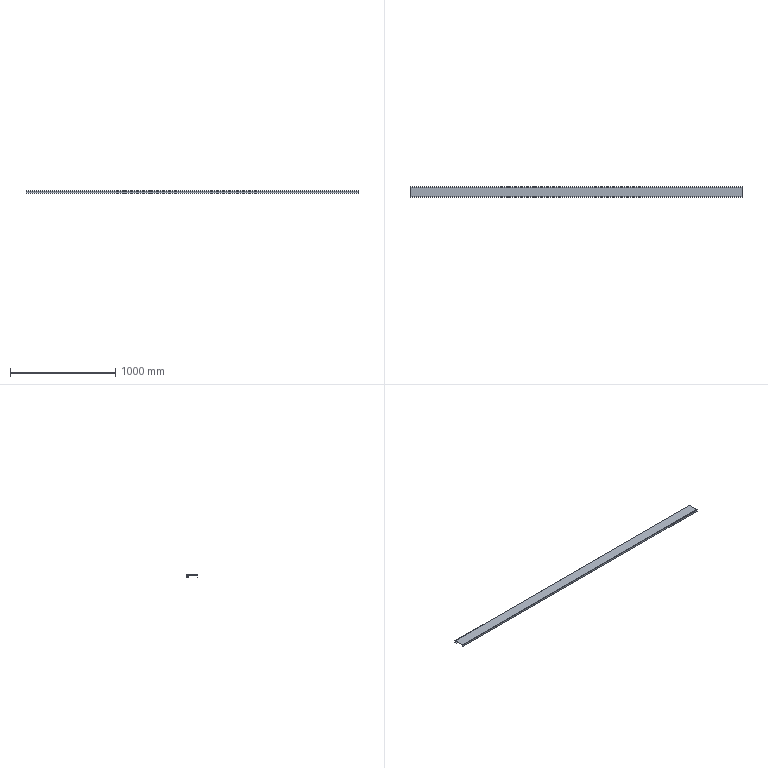Part | STEP file | E3-电柜护栏2踢脚Plate | 1 solid | 18 faces | box 3160 x 100 x 20 mm | volume 726389 mm3 | plane 12 | cylinder 6 | commonest cylinder face diameters 2 x3 5 x3
STEP:
#1=CARTESIAN_POINT('',(0.,0.,0.));
#2=DIRECTION('',(0.,0.,1.));
#3=DIRECTION('',(1.,0.,0.));
#4=AXIS2_PLACEMENT_3D('',#1,#2,#3);
#5=CARTESIAN_POINT('',(-1580.,1.5,-2.5));
#6=VERTEX_POINT('',#5);
#7=CARTESIAN_POINT('',(-1580.,1.5,-20.));
#8=VERTEX_POINT('',#7);
#9=CARTESIAN_POINT('',(-1580.,1.5,-2.5));
#10=DIRECTION('',(0.,0.,-1.));
#11=VECTOR('',#10,1.);
#12=LINE('',#9,#11);
#13=CARTESIAN_POINT('',(1580.,1.5,-2.5));
#14=DIRECTION('',(0.,-1.,0.));
#15=DIRECTION('',(0.,0.,1.));
#16=AXIS2_PLACEMENT_3D('',#13,#14,#15);
#17=PLANE('',#16);
#18=CARTESIAN_POINT('',(0.,3160.));
#19=DIRECTION('',(-1.,0.));
#20=VECTOR('',#19,1.);
#21=LINE('',#18,#20);
#22=(GEOMETRIC_REPRESENTATION_CONTEXT(2)PARAMETRIC_REPRESENTATION_CONTEXT()REPRESENTATION_CONTEXT('',''));
#23=DEFINITIONAL_REPRESENTATION('',(#21),#22);
#24=PCURVE('',#17,#23);
#25=CARTESIAN_POINT('',(-1580.,2.5,-2.5));
#26=DIRECTION('',(-1.,0.,0.));
#27=DIRECTION('',(0.,0.,-1.));
#28=AXIS2_PLACEMENT_3D('',#25,#26,#27);
#29=PLANE('',#28);
#30=CARTESIAN_POINT('',(0.,1.));
#31=DIRECTION('',(1.,0.));
#32=VECTOR('',#31,1.);
#33=LINE('',#30,#32);
#34=(GEOMETRIC_REPRESENTATION_CONTEXT(2)PARAMETRIC_REPRESENTATION_CONTEXT()REPRESENTATION_CONTEXT('',''));
#35=DEFINITIONAL_REPRESENTATION('',(#33),#34);
#36=PCURVE('',#29,#35);
#37=SURFACE_CURVE('',#12,(#24,#36),.PCURVE_S1.);
#38=EDGE_CURVE('',#6,#8,#37,.T.);
#39=ORIENTED_EDGE('',*,*,#38,.F.);
#40=CARTESIAN_POINT('',(1580.,1.5,-2.5));
#41=VERTEX_POINT('',#40);
#42=CARTESIAN_POINT('',(1580.,1.5,-2.5));
#43=DIRECTION('',(-1.,0.,0.));
#44=VECTOR('',#43,1.);
#45=LINE('',#42,#44);
#46=CARTESIAN_POINT('',(0.,0.));
#47=DIRECTION('',(0.,1.));
#48=VECTOR('',#47,1.);
#49=LINE('',#46,#48);
#50=(GEOMETRIC_REPRESENTATION_CONTEXT(2)PARAMETRIC_REPRESENTATION_CONTEXT()REPRESENTATION_CONTEXT('',''));
#51=DEFINITIONAL_REPRESENTATION('',(#49),#50);
#52=PCURVE('',#17,#51);
#53=CARTESIAN_POINT('',(1580.,2.5,-2.5));
#54=DIRECTION('',(-1.,0.,0.));
#55=DIRECTION('',(0.,0.,-1.));
#56=AXIS2_PLACEMENT_3D('',#53,#54,#55);
#57=CYLINDRICAL_SURFACE('',#56,1.);
#58=CARTESIAN_POINT('',(1.571,0.));
#59=DIRECTION('',(0.,1.));
#60=VECTOR('',#59,1.);
#61=LINE('',#58,#60);
#62=(GEOMETRIC_REPRESENTATION_CONTEXT(2)PARAMETRIC_REPRESENTATION_CONTEXT()REPRESENTATION_CONTEXT('',''));
#63=DEFINITIONAL_REPRESENTATION('',(#61),#62);
#64=PCURVE('',#57,#63);
#65=SURFACE_CURVE('',#45,(#52,#64),.PCURVE_S1.);
#66=EDGE_CURVE('',#41,#6,#65,.T.);
#67=ORIENTED_EDGE('',*,*,#66,.F.);
#68=CARTESIAN_POINT('',(1580.,1.5,-20.));
#69=VERTEX_POINT('',#68);
#70=CARTESIAN_POINT('',(1580.,1.5,-2.5));
#71=DIRECTION('',(0.,0.,-1.));
#72=VECTOR('',#71,1.);
#73=LINE('',#70,#72);
#74=CARTESIAN_POINT('',(0.,0.));
#75=DIRECTION('',(-1.,0.));
#76=VECTOR('',#75,1.);
#77=LINE('',#74,#76);
#78=(GEOMETRIC_REPRESENTATION_CONTEXT(2)PARAMETRIC_REPRESENTATION_CONTEXT()REPRESENTATION_CONTEXT('',''));
#79=DEFINITIONAL_REPRESENTATION('',(#77),#78);
#80=PCURVE('',#17,#79);
#81=CARTESIAN_POINT('',(1580.,2.5,-2.5));
#82=DIRECTION('',(-1.,0.,0.));
#83=DIRECTION('',(0.,0.,-1.));
#84=AXIS2_PLACEMENT_3D('',#81,#82,#83);
#85=PLANE('',#84);
#86=CARTESIAN_POINT('',(0.,1.));
#87=DIRECTION('',(1.,0.));
#88=VECTOR('',#87,1.);
#89=LINE('',#86,#88);
#90=(GEOMETRIC_REPRESENTATION_CONTEXT(2)PARAMETRIC_REPRESENTATION_CONTEXT()REPRESENTATION_CONTEXT('',''));
#91=DEFINITIONAL_REPRESENTATION('',(#89),#90);
#92=PCURVE('',#85,#91);
#93=SURFACE_CURVE('',#73,(#80,#92),.PCURVE_S1.);
#94=EDGE_CURVE('',#41,#69,#93,.T.);
#95=ORIENTED_EDGE('',*,*,#94,.T.);
#96=CARTESIAN_POINT('',(1580.,1.5,-20.));
#97=DIRECTION('',(-1.,0.,0.));
#98=VECTOR('',#97,1.);
#99=LINE('',#96,#98);
#100=CARTESIAN_POINT('',(-17.5,0.));
#101=DIRECTION('',(0.,1.));
#102=VECTOR('',#101,1.);
#103=LINE('',#100,#102);
#104=(GEOMETRIC_REPRESENTATION_CONTEXT(2)PARAMETRIC_REPRESENTATION_CONTEXT()REPRESENTATION_CONTEXT('',''));
#105=DEFINITIONAL_REPRESENTATION('',(#103),#104);
#106=PCURVE('',#17,#105);
#107=CARTESIAN_POINT('',(1580.,0.,-20.));
#108=DIRECTION('',(0.,0.,-1.));
#109=DIRECTION('',(1.,0.,0.));
#110=AXIS2_PLACEMENT_3D('',#107,#108,#109);
#111=PLANE('',#110);
#112=CARTESIAN_POINT('',(0.,-1.5));
#113=DIRECTION('',(-1.,0.));
#114=VECTOR('',#113,1.);
#115=LINE('',#112,#114);
#116=(GEOMETRIC_REPRESENTATION_CONTEXT(2)PARAMETRIC_REPRESENTATION_CONTEXT()REPRESENTATION_CONTEXT('',''));
#117=DEFINITIONAL_REPRESENTATION('',(#115),#116);
#118=PCURVE('',#111,#117);
#119=SURFACE_CURVE('',#99,(#106,#118),.PCURVE_S1.);
#120=EDGE_CURVE('',#69,#8,#119,.T.);
#121=ORIENTED_EDGE('',*,*,#120,.T.);
#122=EDGE_LOOP('',(#39,#67,#95,#121));
#123=FACE_BOUND('',#122,.T.);
#124=ADVANCED_FACE('',(#123),#17,.F.);
#125=CARTESIAN_POINT('',(-1580.,0.,-20.));
#126=VERTEX_POINT('',#125);
#127=CARTESIAN_POINT('',(-1580.,0.,-20.));
#128=DIRECTION('',(0.,1.,0.));
#129=VECTOR('',#128,1.);
#130=LINE('',#127,#129);
#131=CARTESIAN_POINT('',(-3160.,0.));
#132=DIRECTION('',(0.,-1.));
#133=VECTOR('',#132,1.);
#134=LINE('',#131,#133);
#135=(GEOMETRIC_REPRESENTATION_CONTEXT(2)PARAMETRIC_REPRESENTATION_CONTEXT()REPRESENTATION_CONTEXT('',''));
#136=DEFINITIONAL_REPRESENTATION('',(#134),#135);
#137=PCURVE('',#111,#136);
#138=CARTESIAN_POINT('',(17.5,2.5));
#139=DIRECTION('',(0.,-1.));
#140=VECTOR('',#139,1.);
#141=LINE('',#138,#140);
#142=(GEOMETRIC_REPRESENTATION_CONTEXT(2)PARAMETRIC_REPRESENTATION_CONTEXT()REPRESENTATION_CONTEXT('',''));
#143=DEFINITIONAL_REPRESENTATION('',(#141),#142);
#144=PCURVE('',#29,#143);
#145=SURFACE_CURVE('',#130,(#137,#144),.PCURVE_S1.);
#146=EDGE_CURVE('',#126,#8,#145,.T.);
#147=ORIENTED_EDGE('',*,*,#146,.T.);
#148=ORIENTED_EDGE('',*,*,#120,.F.);
#149=CARTESIAN_POINT('',(1580.,0.,-20.));
#150=VERTEX_POINT('',#149);
#151=CARTESIAN_POINT('',(1580.,0.,-20.));
#152=DIRECTION('',(0.,1.,0.));
#153=VECTOR('',#152,1.);
#154=LINE('',#151,#153);
#155=CARTESIAN_POINT('',(0.,0.));
#156=DIRECTION('',(0.,-1.));
#157=VECTOR('',#156,1.);
#158=LINE('',#155,#157);
#159=(GEOMETRIC_REPRESENTATION_CONTEXT(2)PARAMETRIC_REPRESENTATION_CONTEXT()REPRESENTATION_CONTEXT('',''));
#160=DEFINITIONAL_REPRESENTATION('',(#158),#159);
#161=PCURVE('',#111,#160);
#162=CARTESIAN_POINT('',(17.5,2.5));
#163=DIRECTION('',(0.,-1.));
#164=VECTOR('',#163,1.);
#165=LINE('',#162,#164);
#166=(GEOMETRIC_REPRESENTATION_CONTEXT(2)PARAMETRIC_REPRESENTATION_CONTEXT()REPRESENTATION_CONTEXT('',''));
#167=DEFINITIONAL_REPRESENTATION('',(#165),#166);
#168=PCURVE('',#85,#167);
#169=SURFACE_CURVE('',#154,(#161,#168),.PCURVE_S1.);
#170=EDGE_CURVE('',#150,#69,#169,.T.);
#171=ORIENTED_EDGE('',*,*,#170,.F.);
#172=CARTESIAN_POINT('',(1580.,0.,-20.));
#173=DIRECTION('',(-1.,0.,0.));
#174=VECTOR('',#173,1.);
#175=LINE('',#172,#174);
#176=CARTESIAN_POINT('',(0.,0.));
#177=DIRECTION('',(-1.,0.));
#178=VECTOR('',#177,1.);
#179=LINE('',#176,#178);
#180=(GEOMETRIC_REPRESENTATION_CONTEXT(2)PARAMETRIC_REPRESENTATION_CONTEXT()REPRESENTATION_CONTEXT('',''));
#181=DEFINITIONAL_REPRESENTATION('',(#179),#180);
#182=PCURVE('',#111,#181);
#183=CARTESIAN_POINT('',(1580.,0.,-2.5));
#184=DIRECTION('',(0.,-1.,0.));
#185=DIRECTION('',(0.,0.,1.));
#186=AXIS2_PLACEMENT_3D('',#183,#184,#185);
#187=PLANE('',#186);
#188=CARTESIAN_POINT('',(-17.5,0.));
#189=DIRECTION('',(0.,1.));
#190=VECTOR('',#189,1.);
#191=LINE('',#188,#190);
#192=(GEOMETRIC_REPRESENTATION_CONTEXT(2)PARAMETRIC_REPRESENTATION_CONTEXT()REPRESENTATION_CONTEXT('',''));
#193=DEFINITIONAL_REPRESENTATION('',(#191),#192);
#194=PCURVE('',#187,#193);
#195=SURFACE_CURVE('',#175,(#182,#194),.PCURVE_S1.);
#196=EDGE_CURVE('',#150,#126,#195,.T.);
#197=ORIENTED_EDGE('',*,*,#196,.T.);
#198=EDGE_LOOP('',(#147,#148,#171,#197));
#199=FACE_BOUND('',#198,.T.);
#200=ADVANCED_FACE('',(#199),#111,.T.);
#201=CARTESIAN_POINT('',(-1580.,0.,-2.5));
#202=VERTEX_POINT('',#201);
#203=CARTESIAN_POINT('',(-1580.,0.,-2.5));
#204=DIRECTION('',(0.,0.,-1.));
#205=VECTOR('',#204,1.);
#206=LINE('',#203,#205);
#207=CARTESIAN_POINT('',(0.,3160.));
#208=DIRECTION('',(-1.,0.));
#209=VECTOR('',#208,1.);
#210=LINE('',#207,#209);
#211=(GEOMETRIC_REPRESENTATION_CONTEXT(2)PARAMETRIC_REPRESENTATION_CONTEXT()REPRESENTATION_CONTEXT('',''));
#212=DEFINITIONAL_REPRESENTATION('',(#210),#211);
#213=PCURVE('',#187,#212);
#214=CARTESIAN_POINT('',(0.,2.5));
#215=DIRECTION('',(1.,0.));
#216=VECTOR('',#215,1.);
#217=LINE('',#214,#216);
#218=(GEOMETRIC_REPRESENTATION_CONTEXT(2)PARAMETRIC_REPRESENTATION_CONTEXT()REPRESENTATION_CONTEXT('',''));
#219=DEFINITIONAL_REPRESENTATION('',(#217),#218);
#220=PCURVE('',#29,#219);
#221=SURFACE_CURVE('',#206,(#213,#220),.PCURVE_S1.);
#222=EDGE_CURVE('',#202,#126,#221,.T.);
#223=ORIENTED_EDGE('',*,*,#222,.T.);
#224=ORIENTED_EDGE('',*,*,#196,.F.);
#225=CARTESIAN_POINT('',(1580.,0.,-2.5));
#226=VERTEX_POINT('',#225);
#227=CARTESIAN_POINT('',(1580.,0.,-2.5));
#228=DIRECTION('',(0.,0.,-1.));
#229=VECTOR('',#228,1.);
#230=LINE('',#227,#229);
#231=CARTESIAN_POINT('',(0.,0.));
#232=DIRECTION('',(-1.,0.));
#233=VECTOR('',#232,1.);
#234=LINE('',#231,#233);
#235=(GEOMETRIC_REPRESENTATION_CONTEXT(2)PARAMETRIC_REPRESENTATION_CONTEXT()REPRESENTATION_CONTEXT('',''));
#236=DEFINITIONAL_REPRESENTATION('',(#234),#235);
#237=PCURVE('',#187,#236);
#238=CARTESIAN_POINT('',(0.,2.5));
#239=DIRECTION('',(1.,0.));
#240=VECTOR('',#239,1.);
#241=LINE('',#238,#240);
#242=(GEOMETRIC_REPRESENTATION_CONTEXT(2)PARAMETRIC_REPRESENTATION_CONTEXT()REPRESENTATION_CONTEXT('',''));
#243=DEFINITIONAL_REPRESENTATION('',(#241),#242);
#244=PCURVE('',#85,#243);
#245=SURFACE_CURVE('',#230,(#237,#244),.PCURVE_S1.);
#246=EDGE_CURVE('',#226,#150,#245,.T.);
#247=ORIENTED_EDGE('',*,*,#246,.F.);
#248=CARTESIAN_POINT('',(1580.,0.,-2.5));
#249=DIRECTION('',(-1.,0.,0.));
#250=VECTOR('',#249,1.);
#251=LINE('',#248,#250);
#252=CARTESIAN_POINT('',(0.,0.));
#253=DIRECTION('',(0.,1.));
#254=VECTOR('',#253,1.);
#255=LINE('',#252,#254);
#256=(GEOMETRIC_REPRESENTATION_CONTEXT(2)PARAMETRIC_REPRESENTATION_CONTEXT()REPRESENTATION_CONTEXT('',''));
#257=DEFINITIONAL_REPRESENTATION('',(#255),#256);
#258=PCURVE('',#187,#257);
#259=CARTESIAN_POINT('',(1580.,2.5,-2.5));
#260=DIRECTION('',(-1.,0.,0.));
#261=DIRECTION('',(0.,0.,-1.));
#262=AXIS2_PLACEMENT_3D('',#259,#260,#261);
#263=CYLINDRICAL_SURFACE('',#262,2.5);
#264=CARTESIAN_POINT('',(1.571,0.));
#265=DIRECTION('',(0.,1.));
#266=VECTOR('',#265,1.);
#267=LINE('',#264,#266);
#268=(GEOMETRIC_REPRESENTATION_CONTEXT(2)PARAMETRIC_REPRESENTATION_CONTEXT()REPRESENTATION_CONTEXT('',''));
#269=DEFINITIONAL_REPRESENTATION('',(#267),#268);
#270=PCURVE('',#263,#269);
#271=SURFACE_CURVE('',#251,(#258,#270),.PCURVE_S1.);
#272=EDGE_CURVE('',#226,#202,#271,.T.);
#273=ORIENTED_EDGE('',*,*,#272,.T.);
#274=EDGE_LOOP('',(#223,#224,#247,#273));
#275=FACE_BOUND('',#274,.T.);
#276=ADVANCED_FACE('',(#275),#187,.T.);
#277=CARTESIAN_POINT('',(-1580.,2.5,0.));
#278=VERTEX_POINT('',#277);
#279=CARTESIAN_POINT('',(-1580.,2.5,-2.5));
#280=DIRECTION('',(1.,0.,0.));
#281=DIRECTION('',(0.,0.,-1.));
#282=AXIS2_PLACEMENT_3D('',#279,#280,#281);
#283=CIRCLE('',#282,2.5);
#284=CARTESIAN_POINT('',(6.283,3160.));
#285=DIRECTION('',(-1.,0.));
#286=VECTOR('',#285,1.);
#287=LINE('',#284,#286);
#288=(GEOMETRIC_REPRESENTATION_CONTEXT(2)PARAMETRIC_REPRESENTATION_CONTEXT()REPRESENTATION_CONTEXT('',''));
#289=DEFINITIONAL_REPRESENTATION('',(#287),#288);
#290=PCURVE('',#263,#289);
#291=CARTESIAN_POINT('',(2.5,0.));
#292=CARTESIAN_POINT('',(2.5,-4.33));
#293=CARTESIAN_POINT('',(-1.25,-2.165));
#294=CARTESIAN_POINT('',(-5.,0.));
#295=CARTESIAN_POINT('',(-1.25,2.165));
#296=CARTESIAN_POINT('',(2.5,4.33));
#297=CARTESIAN_POINT('',(2.5,0.));
#298=(BOUNDED_CURVE()B_SPLINE_CURVE(2,(#291,#292,#293,#294,#295,#296,#297),.UNSPECIFIED.,.T.,.F.)B_SPLINE_CURVE_WITH_KNOTS((1,2,2,2,2,1),(-2.094,0.,2.094,4.189,6.283,8.378),.UNSPECIFIED.)CURVE()GEOMETRIC_REPRESENTATION_ITEM()RATIONAL_B_SPLINE_CURVE((1.,0.5,1.,0.5,1.,0.5,1.))REPRESENTATION_ITEM(''));
#299=(GEOMETRIC_REPRESENTATION_CONTEXT(2)PARAMETRIC_REPRESENTATION_CONTEXT()REPRESENTATION_CONTEXT('',''));
#300=DEFINITIONAL_REPRESENTATION('',(#298),#299);
#301=PCURVE('',#29,#300);
#302=SURFACE_CURVE('',#283,(#290,#301),.PCURVE_S1.);
#303=EDGE_CURVE('',#278,#202,#302,.T.);
#304=ORIENTED_EDGE('',*,*,#303,.T.);
#305=ORIENTED_EDGE('',*,*,#272,.F.);
#306=CARTESIAN_POINT('',(1580.,2.5,0.));
#307=VERTEX_POINT('',#306);
#308=CARTESIAN_POINT('',(1580.,2.5,-2.5));
#309=DIRECTION('',(1.,0.,0.));
#310=DIRECTION('',(0.,0.,-1.));
#311=AXIS2_PLACEMENT_3D('',#308,#309,#310);
#312=CIRCLE('',#311,2.5);
#313=CARTESIAN_POINT('',(6.283,0.));
#314=DIRECTION('',(-1.,0.));
#315=VECTOR('',#314,1.);
#316=LINE('',#313,#315);
#317=(GEOMETRIC_REPRESENTATION_CONTEXT(2)PARAMETRIC_REPRESENTATION_CONTEXT()REPRESENTATION_CONTEXT('',''));
#318=DEFINITIONAL_REPRESENTATION('',(#316),#317);
#319=PCURVE('',#263,#318);
#320=CARTESIAN_POINT('',(2.5,0.));
#321=CARTESIAN_POINT('',(2.5,-4.33));
#322=CARTESIAN_POINT('',(-1.25,-2.165));
#323=CARTESIAN_POINT('',(-5.,0.));
#324=CARTESIAN_POINT('',(-1.25,2.165));
#325=CARTESIAN_POINT('',(2.5,4.33));
#326=CARTESIAN_POINT('',(2.5,0.));
#327=(BOUNDED_CURVE()B_SPLINE_CURVE(2,(#320,#321,#322,#323,#324,#325,#326),.UNSPECIFIED.,.T.,.F.)B_SPLINE_CURVE_WITH_KNOTS((1,2,2,2,2,1),(-2.094,0.,2.094,4.189,6.283,8.378),.UNSPECIFIED.)CURVE()GEOMETRIC_REPRESENTATION_ITEM()RATIONAL_B_SPLINE_CURVE((1.,0.5,1.,0.5,1.,0.5,1.))REPRESENTATION_ITEM(''));
#328=(GEOMETRIC_REPRESENTATION_CONTEXT(2)PARAMETRIC_REPRESENTATION_CONTEXT()REPRESENTATION_CONTEXT('',''));
#329=DEFINITIONAL_REPRESENTATION('',(#327),#328);
#330=PCURVE('',#85,#329);
#331=SURFACE_CURVE('',#312,(#319,#330),.PCURVE_S1.);
#332=EDGE_CURVE('',#307,#226,#331,.T.);
#333=ORIENTED_EDGE('',*,*,#332,.F.);
#334=CARTESIAN_POINT('',(1580.,2.5,0.));
#335=DIRECTION('',(-1.,0.,0.));
#336=VECTOR('',#335,1.);
#337=LINE('',#334,#336);
#338=CARTESIAN_POINT('',(3.142,0.));
#339=DIRECTION('',(0.,1.));
#340=VECTOR('',#339,1.);
#341=LINE('',#338,#340);
#342=(GEOMETRIC_REPRESENTATION_CONTEXT(2)PARAMETRIC_REPRESENTATION_CONTEXT()REPRESENTATION_CONTEXT('',''));
#343=DEFINITIONAL_REPRESENTATION('',(#341),#342);
#344=PCURVE('',#263,#343);
#345=CARTESIAN_POINT('',(1580.,2.5,0.));
#346=DIRECTION('',(0.,0.,1.));
#347=DIRECTION('',(-1.,0.,0.));
#348=AXIS2_PLACEMENT_3D('',#345,#346,#347);
#349=PLANE('',#348);
#350=CARTESIAN_POINT('',(0.,0.));
#351=DIRECTION('',(1.,0.));
#352=VECTOR('',#351,1.);
#353=LINE('',#350,#352);
#354=(GEOMETRIC_REPRESENTATION_CONTEXT(2)PARAMETRIC_REPRESENTATION_CONTEXT()REPRESENTATION_CONTEXT('',''));
#355=DEFINITIONAL_REPRESENTATION('',(#353),#354);
#356=PCURVE('',#349,#355);
#357=SURFACE_CURVE('',#337,(#344,#356),.PCURVE_S1.);
#358=EDGE_CURVE('',#307,#278,#357,.T.);
#359=ORIENTED_EDGE('',*,*,#358,.T.);
#360=EDGE_LOOP('',(#304,#305,#333,#359));
#361=FACE_BOUND('',#360,.T.);
#362=ADVANCED_FACE('',(#361),#263,.T.);
#363=CARTESIAN_POINT('',(-1580.,97.5,0.));
#364=VERTEX_POINT('',#363);
#365=CARTESIAN_POINT('',(-1580.,2.5,0.));
#366=DIRECTION('',(0.,-1.,0.));
#367=VECTOR('',#366,1.);
#368=LINE('',#365,#367);
#369=CARTESIAN_POINT('',(3160.,0.));
#370=DIRECTION('',(0.,1.));
#371=VECTOR('',#370,1.);
#372=LINE('',#369,#371);
#373=(GEOMETRIC_REPRESENTATION_CONTEXT(2)PARAMETRIC_REPRESENTATION_CONTEXT()REPRESENTATION_CONTEXT('',''));
#374=DEFINITIONAL_REPRESENTATION('',(#372),#373);
#375=PCURVE('',#349,#374);
#376=CARTESIAN_POINT('',(-2.5,0.));
#377=DIRECTION('',(0.,1.));
#378=VECTOR('',#377,1.);
#379=LINE('',#376,#378);
#380=(GEOMETRIC_REPRESENTATION_CONTEXT(2)PARAMETRIC_REPRESENTATION_CONTEXT()REPRESENTATION_CONTEXT('',''));
#381=DEFINITIONAL_REPRESENTATION('',(#379),#380);
#382=PCURVE('',#29,#381);
#383=SURFACE_CURVE('',#368,(#375,#382),.PCURVE_S1.);
#384=EDGE_CURVE('',#364,#278,#383,.T.);
#385=ORIENTED_EDGE('',*,*,#384,.T.);
#386=ORIENTED_EDGE('',*,*,#358,.F.);
#387=CARTESIAN_POINT('',(1580.,97.5,0.));
#388=VERTEX_POINT('',#387);
#389=CARTESIAN_POINT('',(1580.,2.5,0.));
#390=DIRECTION('',(0.,-1.,0.));
#391=VECTOR('',#390,1.);
#392=LINE('',#389,#391);
#393=CARTESIAN_POINT('',(0.,0.));
#394=DIRECTION('',(0.,1.));
#395=VECTOR('',#394,1.);
#396=LINE('',#393,#395);
#397=(GEOMETRIC_REPRESENTATION_CONTEXT(2)PARAMETRIC_REPRESENTATION_CONTEXT()REPRESENTATION_CONTEXT('',''));
#398=DEFINITIONAL_REPRESENTATION('',(#396),#397);
#399=PCURVE('',#349,#398);
#400=CARTESIAN_POINT('',(-2.5,0.));
#401=DIRECTION('',(0.,1.));
#402=VECTOR('',#401,1.);
#403=LINE('',#400,#402);
#404=(GEOMETRIC_REPRESENTATION_CONTEXT(2)PARAMETRIC_REPRESENTATION_CONTEXT()REPRESENTATION_CONTEXT('',''));
#405=DEFINITIONAL_REPRESENTATION('',(#403),#404);
#406=PCURVE('',#85,#405);
#407=SURFACE_CURVE('',#392,(#399,#406),.PCURVE_S1.);
#408=EDGE_CURVE('',#388,#307,#407,.T.);
#409=ORIENTED_EDGE('',*,*,#408,.F.);
#410=CARTESIAN_POINT('',(1580.,97.5,0.));
#411=DIRECTION('',(-1.,0.,0.));
#412=VECTOR('',#411,1.);
#413=LINE('',#410,#412);
#414=CARTESIAN_POINT('',(0.,-95.));
#415=DIRECTION('',(1.,0.));
#416=VECTOR('',#415,1.);
#417=LINE('',#414,#416);
#418=(GEOMETRIC_REPRESENTATION_CONTEXT(2)PARAMETRIC_REPRESENTATION_CONTEXT()REPRESENTATION_CONTEXT('',''));
#419=DEFINITIONAL_REPRESENTATION('',(#417),#418);
#420=PCURVE('',#349,#419);
#421=CARTESIAN_POINT('',(1580.,97.5,-2.5));
#422=DIRECTION('',(-1.,0.,0.));
#423=DIRECTION('',(0.,0.,-1.));
#424=AXIS2_PLACEMENT_3D('',#421,#422,#423);
#425=CYLINDRICAL_SURFACE('',#424,2.5);
#426=CARTESIAN_POINT('',(3.142,0.));
#427=DIRECTION('',(0.,1.));
#428=VECTOR('',#427,1.);
#429=LINE('',#426,#428);
#430=(GEOMETRIC_REPRESENTATION_CONTEXT(2)PARAMETRIC_REPRESENTATION_CONTEXT()REPRESENTATION_CONTEXT('',''));
#431=DEFINITIONAL_REPRESENTATION('',(#429),#430);
#432=PCURVE('',#425,#431);
#433=SURFACE_CURVE('',#413,(#420,#432),.PCURVE_S1.);
#434=EDGE_CURVE('',#388,#364,#433,.T.);
#435=ORIENTED_EDGE('',*,*,#434,.T.);
#436=EDGE_LOOP('',(#385,#386,#409,#435));
#437=FACE_BOUND('',#436,.T.);
#438=ADVANCED_FACE('',(#437),#349,.T.);
#439=CARTESIAN_POINT('',(-1580.,100.,-2.5));
#440=VERTEX_POINT('',#439);
#441=CARTESIAN_POINT('',(-1580.,97.5,-2.5));
#442=DIRECTION('',(1.,0.,0.));
#443=DIRECTION('',(0.,0.,1.));
#444=AXIS2_PLACEMENT_3D('',#441,#442,#443);
#445=CIRCLE('',#444,2.5);
#446=CARTESIAN_POINT('',(9.425,3160.));
#447=DIRECTION('',(-1.,0.));
#448=VECTOR('',#447,1.);
#449=LINE('',#446,#448);
#450=(GEOMETRIC_REPRESENTATION_CONTEXT(2)PARAMETRIC_REPRESENTATION_CONTEXT()REPRESENTATION_CONTEXT('',''));
#451=DEFINITIONAL_REPRESENTATION('',(#449),#450);
#452=PCURVE('',#425,#451);
#453=CARTESIAN_POINT('',(-2.5,-95.));
#454=CARTESIAN_POINT('',(-2.5,-90.67));
#455=CARTESIAN_POINT('',(1.25,-92.835));
#456=CARTESIAN_POINT('',(5.,-95.));
#457=CARTESIAN_POINT('',(1.25,-97.165));
#458=CARTESIAN_POINT('',(-2.5,-99.33));
#459=CARTESIAN_POINT('',(-2.5,-95.));
#460=(BOUNDED_CURVE()B_SPLINE_CURVE(2,(#453,#454,#455,#456,#457,#458,#459),.UNSPECIFIED.,.T.,.F.)B_SPLINE_CURVE_WITH_KNOTS((1,2,2,2,2,1),(-2.094,0.,2.094,4.189,6.283,8.378),.UNSPECIFIED.)CURVE()GEOMETRIC_REPRESENTATION_ITEM()RATIONAL_B_SPLINE_CURVE((1.,0.5,1.,0.5,1.,0.5,1.))REPRESENTATION_ITEM(''));
#461=(GEOMETRIC_REPRESENTATION_CONTEXT(2)PARAMETRIC_REPRESENTATION_CONTEXT()REPRESENTATION_CONTEXT('',''));
#462=DEFINITIONAL_REPRESENTATION('',(#460),#461);
#463=PCURVE('',#29,#462);
#464=SURFACE_CURVE('',#445,(#452,#463),.PCURVE_S1.);
#465=EDGE_CURVE('',#440,#364,#464,.T.);
#466=ORIENTED_EDGE('',*,*,#465,.T.);
#467=ORIENTED_EDGE('',*,*,#434,.F.);
#468=CARTESIAN_POINT('',(1580.,100.,-2.5));
#469=VERTEX_POINT('',#468);
#470=CARTESIAN_POINT('',(1580.,97.5,-2.5));
#471=DIRECTION('',(1.,0.,0.));
#472=DIRECTION('',(0.,0.,1.));
#473=AXIS2_PLACEMENT_3D('',#470,#471,#472);
#474=CIRCLE('',#473,2.5);
#475=CARTESIAN_POINT('',(9.425,0.));
#476=DIRECTION('',(-1.,0.));
#477=VECTOR('',#476,1.);
#478=LINE('',#475,#477);
#479=(GEOMETRIC_REPRESENTATION_CONTEXT(2)PARAMETRIC_REPRESENTATION_CONTEXT()REPRESENTATION_CONTEXT('',''));
#480=DEFINITIONAL_REPRESENTATION('',(#478),#479);
#481=PCURVE('',#425,#480);
#482=CARTESIAN_POINT('',(-2.5,-95.));
#483=CARTESIAN_POINT('',(-2.5,-90.67));
#484=CARTESIAN_POINT('',(1.25,-92.835));
#485=CARTESIAN_POINT('',(5.,-95.));
#486=CARTESIAN_POINT('',(1.25,-97.165));
#487=CARTESIAN_POINT('',(-2.5,-99.33));
#488=CARTESIAN_POINT('',(-2.5,-95.));
#489=(BOUNDED_CURVE()B_SPLINE_CURVE(2,(#482,#483,#484,#485,#486,#487,#488),.UNSPECIFIED.,.T.,.F.)B_SPLINE_CURVE_WITH_KNOTS((1,2,2,2,2,1),(-2.094,0.,2.094,4.189,6.283,8.378),.UNSPECIFIED.)CURVE()GEOMETRIC_REPRESENTATION_ITEM()RATIONAL_B_SPLINE_CURVE((1.,0.5,1.,0.5,1.,0.5,1.))REPRESENTATION_ITEM(''));
#490=(GEOMETRIC_REPRESENTATION_CONTEXT(2)PARAMETRIC_REPRESENTATION_CONTEXT()REPRESENTATION_CONTEXT('',''));
#491=DEFINITIONAL_REPRESENTATION('',(#489),#490);
#492=PCURVE('',#85,#491);
#493=SURFACE_CURVE('',#474,(#481,#492),.PCURVE_S1.);
#494=EDGE_CURVE('',#469,#388,#493,.T.);
#495=ORIENTED_EDGE('',*,*,#494,.F.);
#496=CARTESIAN_POINT('',(1580.,100.,-2.5));
#497=DIRECTION('',(-1.,0.,0.));
#498=VECTOR('',#497,1.);
#499=LINE('',#496,#498);
#500=CARTESIAN_POINT('',(4.712,0.));
#501=DIRECTION('',(0.,1.));
#502=VECTOR('',#501,1.);
#503=LINE('',#500,#502);
#504=(GEOMETRIC_REPRESENTATION_CONTEXT(2)PARAMETRIC_REPRESENTATION_CONTEXT()REPRESENTATION_CONTEXT('',''));
#505=DEFINITIONAL_REPRESENTATION('',(#503),#504);
#506=PCURVE('',#425,#505);
#507=CARTESIAN_POINT('',(1580.,100.,-2.5));
#508=DIRECTION('',(0.,1.,0.));
#509=DIRECTION('',(0.,0.,-1.));
#510=AXIS2_PLACEMENT_3D('',#507,#508,#509);
#511=PLANE('',#510);
#512=CARTESIAN_POINT('',(0.,0.));
#513=DIRECTION('',(0.,1.));
#514=VECTOR('',#513,1.);
#515=LINE('',#512,#514);
#516=(GEOMETRIC_REPRESENTATION_CONTEXT(2)PARAMETRIC_REPRESENTATION_CONTEXT()REPRESENTATION_CONTEXT('',''));
#517=DEFINITIONAL_REPRESENTATION('',(#515),#516);
#518=PCURVE('',#511,#517);
#519=SURFACE_CURVE('',#499,(#506,#518),.PCURVE_S1.);
#520=EDGE_CURVE('',#469,#440,#519,.T.);
#521=ORIENTED_EDGE('',*,*,#520,.T.);
#522=EDGE_LOOP('',(#466,#467,#495,#521));
#523=FACE_BOUND('',#522,.T.);
#524=ADVANCED_FACE('',(#523),#425,.T.);
#525=CARTESIAN_POINT('',(-1580.,100.,-17.5));
#526=VERTEX_POINT('',#525);
#527=CARTESIAN_POINT('',(-1580.,100.,-2.5));
#528=DIRECTION('',(0.,0.,1.));
#529=VECTOR('',#528,1.);
#530=LINE('',#527,#529);
#531=CARTESIAN_POINT('',(0.,3160.));
#532=DIRECTION('',(-1.,0.));
#533=VECTOR('',#532,1.);
#534=LINE('',#531,#533);
#535=(GEOMETRIC_REPRESENTATION_CONTEXT(2)PARAMETRIC_REPRESENTATION_CONTEXT()REPRESENTATION_CONTEXT('',''));
#536=DEFINITIONAL_REPRESENTATION('',(#534),#535);
#537=PCURVE('',#511,#536);
#538=CARTESIAN_POINT('',(0.,-97.5));
#539=DIRECTION('',(-1.,0.));
#540=VECTOR('',#539,1.);
#541=LINE('',#538,#540);
#542=(GEOMETRIC_REPRESENTATION_CONTEXT(2)PARAMETRIC_REPRESENTATION_CONTEXT()REPRESENTATION_CONTEXT('',''));
#543=DEFINITIONAL_REPRESENTATION('',(#541),#542);
#544=PCURVE('',#29,#543);
#545=SURFACE_CURVE('',#530,(#537,#544),.PCURVE_S1.);
#546=EDGE_CURVE('',#526,#440,#545,.T.);
#547=ORIENTED_EDGE('',*,*,#546,.T.);
#548=ORIENTED_EDGE('',*,*,#520,.F.);
#549=CARTESIAN_POINT('',(1580.,100.,-17.5));
#550=VERTEX_POINT('',#549);
#551=CARTESIAN_POINT('',(1580.,100.,-2.5));
#552=DIRECTION('',(0.,0.,1.));
#553=VECTOR('',#552,1.);
#554=LINE('',#551,#553);
#555=CARTESIAN_POINT('',(0.,0.));
#556=DIRECTION('',(-1.,0.));
#557=VECTOR('',#556,1.);
#558=LINE('',#555,#557);
#559=(GEOMETRIC_REPRESENTATION_CONTEXT(2)PARAMETRIC_REPRESENTATION_CONTEXT()REPRESENTATION_CONTEXT('',''));
#560=DEFINITIONAL_REPRESENTATION('',(#558),#559);
#561=PCURVE('',#511,#560);
#562=CARTESIAN_POINT('',(0.,-97.5));
#563=DIRECTION('',(-1.,0.));
#564=VECTOR('',#563,1.);
#565=LINE('',#562,#564);
#566=(GEOMETRIC_REPRESENTATION_CONTEXT(2)PARAMETRIC_REPRESENTATION_CONTEXT()REPRESENTATION_CONTEXT('',''));
#567=DEFINITIONAL_REPRESENTATION('',(#565),#566);
#568=PCURVE('',#85,#567);
#569=SURFACE_CURVE('',#554,(#561,#568),.PCURVE_S1.);
#570=EDGE_CURVE('',#550,#469,#569,.T.);
#571=ORIENTED_EDGE('',*,*,#570,.F.);
#572=CARTESIAN_POINT('',(1580.,100.,-17.5));
#573=DIRECTION('',(-1.,0.,0.));
#574=VECTOR('',#573,1.);
#575=LINE('',#572,#574);
#576=CARTESIAN_POINT('',(15.,0.));
#577=DIRECTION('',(0.,1.));
#578=VECTOR('',#577,1.);
#579=LINE('',#576,#578);
#580=(GEOMETRIC_REPRESENTATION_CONTEXT(2)PARAMETRIC_REPRESENTATION_CONTEXT()REPRESENTATION_CONTEXT('',''));
#581=DEFINITIONAL_REPRESENTATION('',(#579),#580);
#582=PCURVE('',#511,#581);
#583=CARTESIAN_POINT('',(1580.,97.5,-17.5));
#584=DIRECTION('',(-1.,0.,0.));
#585=DIRECTION('',(0.,0.,-1.));
#586=AXIS2_PLACEMENT_3D('',#583,#584,#585);
#587=CYLINDRICAL_SURFACE('',#586,2.5);
#588=CARTESIAN_POINT('',(4.712,0.));
#589=DIRECTION('',(0.,1.));
#590=VECTOR('',#589,1.);
#591=LINE('',#588,#590);
#592=(GEOMETRIC_REPRESENTATION_CONTEXT(2)PARAMETRIC_REPRESENTATION_CONTEXT()REPRESENTATION_CONTEXT('',''));
#593=DEFINITIONAL_REPRESENTATION('',(#591),#592);
#594=PCURVE('',#587,#593);
#595=SURFACE_CURVE('',#575,(#582,#594),.PCURVE_S1.);
#596=EDGE_CURVE('',#550,#526,#595,.T.);
#597=ORIENTED_EDGE('',*,*,#596,.T.);
#598=EDGE_LOOP('',(#547,#548,#571,#597));
#599=FACE_BOUND('',#598,.T.);
#600=ADVANCED_FACE('',(#599),#511,.T.);
#601=CARTESIAN_POINT('',(-1580.,97.5,-20.));
#602=VERTEX_POINT('',#601);
#603=CARTESIAN_POINT('',(-1580.,97.5,-17.5));
#604=DIRECTION('',(1.,0.,0.));
#605=DIRECTION('',(0.,0.,1.));
#606=AXIS2_PLACEMENT_3D('',#603,#604,#605);
#607=CIRCLE('',#606,2.5);
#608=CARTESIAN_POINT('',(9.425,3160.));
#609=DIRECTION('',(-1.,0.));
#610=VECTOR('',#609,1.);
#611=LINE('',#608,#610);
#612=(GEOMETRIC_REPRESENTATION_CONTEXT(2)PARAMETRIC_REPRESENTATION_CONTEXT()REPRESENTATION_CONTEXT('',''));
#613=DEFINITIONAL_REPRESENTATION('',(#611),#612);
#614=PCURVE('',#587,#613);
#615=CARTESIAN_POINT('',(12.5,-95.));
#616=CARTESIAN_POINT('',(12.5,-90.67));
#617=CARTESIAN_POINT('',(16.25,-92.835));
#618=CARTESIAN_POINT('',(20.,-95.));
#619=CARTESIAN_POINT('',(16.25,-97.165));
#620=CARTESIAN_POINT('',(12.5,-99.33));
#621=CARTESIAN_POINT('',(12.5,-95.));
#622=(BOUNDED_CURVE()B_SPLINE_CURVE(2,(#615,#616,#617,#618,#619,#620,#621),.UNSPECIFIED.,.T.,.F.)B_SPLINE_CURVE_WITH_KNOTS((1,2,2,2,2,1),(-2.094,0.,2.094,4.189,6.283,8.378),.UNSPECIFIED.)CURVE()GEOMETRIC_REPRESENTATION_ITEM()RATIONAL_B_SPLINE_CURVE((1.,0.5,1.,0.5,1.,0.5,1.))REPRESENTATION_ITEM(''));
#623=(GEOMETRIC_REPRESENTATION_CONTEXT(2)PARAMETRIC_REPRESENTATION_CONTEXT()REPRESENTATION_CONTEXT('',''));
#624=DEFINITIONAL_REPRESENTATION('',(#622),#623);
#625=PCURVE('',#29,#624);
#626=SURFACE_CURVE('',#607,(#614,#625),.PCURVE_S1.);
#627=EDGE_CURVE('',#602,#526,#626,.T.);
#628=ORIENTED_EDGE('',*,*,#627,.T.);
#629=ORIENTED_EDGE('',*,*,#596,.F.);
#630=CARTESIAN_POINT('',(1580.,97.5,-20.));
#631=VERTEX_POINT('',#630);
#632=CARTESIAN_POINT('',(1580.,97.5,-17.5));
#633=DIRECTION('',(1.,0.,0.));
#634=DIRECTION('',(0.,0.,1.));
#635=AXIS2_PLACEMENT_3D('',#632,#633,#634);
#636=CIRCLE('',#635,2.5);
#637=CARTESIAN_POINT('',(9.425,0.));
#638=DIRECTION('',(-1.,0.));
#639=VECTOR('',#638,1.);
#640=LINE('',#637,#639);
#641=(GEOMETRIC_REPRESENTATION_CONTEXT(2)PARAMETRIC_REPRESENTATION_CONTEXT()REPRESENTATION_CONTEXT('',''));
#642=DEFINITIONAL_REPRESENTATION('',(#640),#641);
#643=PCURVE('',#587,#642);
#644=CARTESIAN_POINT('',(12.5,-95.));
#645=CARTESIAN_POINT('',(12.5,-90.67));
#646=CARTESIAN_POINT('',(16.25,-92.835));
#647=CARTESIAN_POINT('',(20.,-95.));
#648=CARTESIAN_POINT('',(16.25,-97.165));
#649=CARTESIAN_POINT('',(12.5,-99.33));
#650=CARTESIAN_POINT('',(12.5,-95.));
#651=(BOUNDED_CURVE()B_SPLINE_CURVE(2,(#644,#645,#646,#647,#648,#649,#650),.UNSPECIFIED.,.T.,.F.)B_SPLINE_CURVE_WITH_KNOTS((1,2,2,2,2,1),(-2.094,0.,2.094,4.189,6.283,8.378),.UNSPECIFIED.)CURVE()GEOMETRIC_REPRESENTATION_ITEM()RATIONAL_B_SPLINE_CURVE((1.,0.5,1.,0.5,1.,0.5,1.))REPRESENTATION_ITEM(''));
#652=(GEOMETRIC_REPRESENTATION_CONTEXT(2)PARAMETRIC_REPRESENTATION_CONTEXT()REPRESENTATION_CONTEXT('',''));
#653=DEFINITIONAL_REPRESENTATION('',(#651),#652);
#654=PCURVE('',#85,#653);
#655=SURFACE_CURVE('',#636,(#643,#654),.PCURVE_S1.);
#656=EDGE_CURVE('',#631,#550,#655,.T.);
#657=ORIENTED_EDGE('',*,*,#656,.F.);
#658=CARTESIAN_POINT('',(1580.,97.5,-20.));
#659=DIRECTION('',(-1.,0.,0.));
#660=VECTOR('',#659,1.);
#661=LINE('',#658,#660);
#662=CARTESIAN_POINT('',(6.283,0.));
#663=DIRECTION('',(0.,1.));
#664=VECTOR('',#663,1.);
#665=LINE('',#662,#664);
#666=(GEOMETRIC_REPRESENTATION_CONTEXT(2)PARAMETRIC_REPRESENTATION_CONTEXT()REPRESENTATION_CONTEXT('',''));
#667=DEFINITIONAL_REPRESENTATION('',(#665),#666);
#668=PCURVE('',#587,#667);
#669=CARTESIAN_POINT('',(1580.,97.5,-20.));
#670=DIRECTION('',(0.,0.,-1.));
#671=DIRECTION('',(1.,0.,0.));
#672=AXIS2_PLACEMENT_3D('',#669,#670,#671);
#673=PLANE('',#672);
#674=CARTESIAN_POINT('',(0.,0.));
#675=DIRECTION('',(-1.,0.));
#676=VECTOR('',#675,1.);
#677=LINE('',#674,#676);
#678=(GEOMETRIC_REPRESENTATION_CONTEXT(2)PARAMETRIC_REPRESENTATION_CONTEXT()REPRESENTATION_CONTEXT('',''));
#679=DEFINITIONAL_REPRESENTATION('',(#677),#678);
#680=PCURVE('',#673,#679);
#681=SURFACE_CURVE('',#661,(#668,#680),.PCURVE_S1.);
#682=EDGE_CURVE('',#631,#602,#681,.T.);
#683=ORIENTED_EDGE('',*,*,#682,.T.);
#684=EDGE_LOOP('',(#628,#629,#657,#683));
#685=FACE_BOUND('',#684,.T.);
#686=ADVANCED_FACE('',(#685),#587,.T.);
#687=CARTESIAN_POINT('',(-1580.,80.,-20.));
#688=VERTEX_POINT('',#687);
#689=CARTESIAN_POINT('',(-1580.,97.5,-20.));
#690=DIRECTION('',(0.,1.,0.));
#691=VECTOR('',#690,1.);
#692=LINE('',#689,#691);
#693=CARTESIAN_POINT('',(-3160.,0.));
#694=DIRECTION('',(0.,-1.));
#695=VECTOR('',#694,1.);
#696=LINE('',#693,#695);
#697=(GEOMETRIC_REPRESENTATION_CONTEXT(2)PARAMETRIC_REPRESENTATION_CONTEXT()REPRESENTATION_CONTEXT('',''));
#698=DEFINITIONAL_REPRESENTATION('',(#696),#697);
#699=PCURVE('',#673,#698);
#700=CARTESIAN_POINT('',(17.5,-95.));
#701=DIRECTION('',(0.,-1.));
#702=VECTOR('',#701,1.);
#703=LINE('',#700,#702);
#704=(GEOMETRIC_REPRESENTATION_CONTEXT(2)PARAMETRIC_REPRESENTATION_CONTEXT()REPRESENTATION_CONTEXT('',''));
#705=DEFINITIONAL_REPRESENTATION('',(#703),#704);
#706=PCURVE('',#29,#705);
#707=SURFACE_CURVE('',#692,(#699,#706),.PCURVE_S1.);
#708=EDGE_CURVE('',#688,#602,#707,.T.);
#709=ORIENTED_EDGE('',*,*,#708,.T.);
#710=ORIENTED_EDGE('',*,*,#682,.F.);
#711=CARTESIAN_POINT('',(1580.,80.,-20.));
#712=VERTEX_POINT('',#711);
#713=CARTESIAN_POINT('',(1580.,97.5,-20.));
#714=DIRECTION('',(0.,1.,0.));
#715=VECTOR('',#714,1.);
#716=LINE('',#713,#715);
#717=CARTESIAN_POINT('',(0.,0.));
#718=DIRECTION('',(0.,-1.));
#719=VECTOR('',#718,1.);
#720=LINE('',#717,#719);
#721=(GEOMETRIC_REPRESENTATION_CONTEXT(2)PARAMETRIC_REPRESENTATION_CONTEXT()REPRESENTATION_CONTEXT('',''));
#722=DEFINITIONAL_REPRESENTATION('',(#720),#721);
#723=PCURVE('',#673,#722);
#724=CARTESIAN_POINT('',(17.5,-95.));
#725=DIRECTION('',(0.,-1.));
#726=VECTOR('',#725,1.);
#727=LINE('',#724,#726);
#728=(GEOMETRIC_REPRESENTATION_CONTEXT(2)PARAMETRIC_REPRESENTATION_CONTEXT()REPRESENTATION_CONTEXT('',''));
#729=DEFINITIONAL_REPRESENTATION('',(#727),#728);
#730=PCURVE('',#85,#729);
#731=SURFACE_CURVE('',#716,(#723,#730),.PCURVE_S1.);
#732=EDGE_CURVE('',#712,#631,#731,.T.);
#733=ORIENTED_EDGE('',*,*,#732,.F.);
#734=CARTESIAN_POINT('',(1580.,80.,-20.));
#735=DIRECTION('',(-1.,0.,0.));
#736=VECTOR('',#735,1.);
#737=LINE('',#734,#736);
#738=CARTESIAN_POINT('',(0.,17.5));
#739=DIRECTION('',(-1.,0.));
#740=VECTOR('',#739,1.);
#741=LINE('',#738,#740);
#742=(GEOMETRIC_REPRESENTATION_CONTEXT(2)PARAMETRIC_REPRESENTATION_CONTEXT()REPRESENTATION_CONTEXT('',''));
#743=DEFINITIONAL_REPRESENTATION('',(#741),#742);
#744=PCURVE('',#673,#743);
#745=CARTESIAN_POINT('',(1580.,80.,-18.5));
#746=DIRECTION('',(0.,-1.,0.));
#747=DIRECTION('',(0.,0.,1.));
#748=AXIS2_PLACEMENT_3D('',#745,#746,#747);
#749=PLANE('',#748);
#750=CARTESIAN_POINT('',(-1.5,0.));
#751=DIRECTION('',(0.,1.));
#752=VECTOR('',#751,1.);
#753=LINE('',#750,#752);
#754=(GEOMETRIC_REPRESENTATION_CONTEXT(2)PARAMETRIC_REPRESENTATION_CONTEXT()REPRESENTATION_CONTEXT('',''));
#755=DEFINITIONAL_REPRESENTATION('',(#753),#754);
#756=PCURVE('',#749,#755);
#757=SURFACE_CURVE('',#737,(#744,#756),.PCURVE_S1.);
#758=EDGE_CURVE('',#712,#688,#757,.T.);
#759=ORIENTED_EDGE('',*,*,#758,.T.);
#760=EDGE_LOOP('',(#709,#710,#733,#759));
#761=FACE_BOUND('',#760,.T.);
#762=ADVANCED_FACE('',(#761),#673,.T.);
#763=CARTESIAN_POINT('',(-1580.,80.,-18.5));
#764=VERTEX_POINT('',#763);
#765=CARTESIAN_POINT('',(-1580.,80.,-18.5));
#766=DIRECTION('',(0.,0.,-1.));
#767=VECTOR('',#766,1.);
#768=LINE('',#765,#767);
#769=CARTESIAN_POINT('',(0.,3160.));
#770=DIRECTION('',(-1.,0.));
#771=VECTOR('',#770,1.);
#772=LINE('',#769,#771);
#773=(GEOMETRIC_REPRESENTATION_CONTEXT(2)PARAMETRIC_REPRESENTATION_CONTEXT()REPRESENTATION_CONTEXT('',''));
#774=DEFINITIONAL_REPRESENTATION('',(#772),#773);
#775=PCURVE('',#749,#774);
#776=CARTESIAN_POINT('',(16.,-77.5));
#777=DIRECTION('',(1.,0.));
#778=VECTOR('',#777,1.);
#779=LINE('',#776,#778);
#780=(GEOMETRIC_REPRESENTATION_CONTEXT(2)PARAMETRIC_REPRESENTATION_CONTEXT()REPRESENTATION_CONTEXT('',''));
#781=DEFINITIONAL_REPRESENTATION('',(#779),#780);
#782=PCURVE('',#29,#781);
#783=SURFACE_CURVE('',#768,(#775,#782),.PCURVE_S1.);
#784=EDGE_CURVE('',#764,#688,#783,.T.);
#785=ORIENTED_EDGE('',*,*,#784,.T.);
#786=ORIENTED_EDGE('',*,*,#758,.F.);
#787=CARTESIAN_POINT('',(1580.,80.,-18.5));
#788=VERTEX_POINT('',#787);
#789=CARTESIAN_POINT('',(1580.,80.,-18.5));
#790=DIRECTION('',(0.,0.,-1.));
#791=VECTOR('',#790,1.);
#792=LINE('',#789,#791);
#793=CARTESIAN_POINT('',(0.,0.));
#794=DIRECTION('',(-1.,0.));
#795=VECTOR('',#794,1.);
#796=LINE('',#793,#795);
#797=(GEOMETRIC_REPRESENTATION_CONTEXT(2)PARAMETRIC_REPRESENTATION_CONTEXT()REPRESENTATION_CONTEXT('',''));
#798=DEFINITIONAL_REPRESENTATION('',(#796),#797);
#799=PCURVE('',#749,#798);
#800=CARTESIAN_POINT('',(16.,-77.5));
#801=DIRECTION('',(1.,0.));
#802=VECTOR('',#801,1.);
#803=LINE('',#800,#802);
#804=(GEOMETRIC_REPRESENTATION_CONTEXT(2)PARAMETRIC_REPRESENTATION_CONTEXT()REPRESENTATION_CONTEXT('',''));
#805=DEFINITIONAL_REPRESENTATION('',(#803),#804);
#806=PCURVE('',#85,#805);
#807=SURFACE_CURVE('',#792,(#799,#806),.PCURVE_S1.);
#808=EDGE_CURVE('',#788,#712,#807,.T.);
#809=ORIENTED_EDGE('',*,*,#808,.F.);
#810=CARTESIAN_POINT('',(1580.,80.,-18.5));
#811=DIRECTION('',(-1.,0.,0.));
#812=VECTOR('',#811,1.);
#813=LINE('',#810,#812);
#814=CARTESIAN_POINT('',(0.,0.));
#815=DIRECTION('',(0.,1.));
#816=VECTOR('',#815,1.);
#817=LINE('',#814,#816);
#818=(GEOMETRIC_REPRESENTATION_CONTEXT(2)PARAMETRIC_REPRESENTATION_CONTEXT()REPRESENTATION_CONTEXT('',''));
#819=DEFINITIONAL_REPRESENTATION('',(#817),#818);
#820=PCURVE('',#749,#819);
#821=CARTESIAN_POINT('',(1580.,97.5,-18.5));
#822=DIRECTION('',(0.,0.,-1.));
#823=DIRECTION('',(1.,0.,0.));
#824=AXIS2_PLACEMENT_3D('',#821,#822,#823);
#825=PLANE('',#824);
#826=CARTESIAN_POINT('',(0.,17.5));
#827=DIRECTION('',(-1.,0.));
#828=VECTOR('',#827,1.);
#829=LINE('',#826,#828);
#830=(GEOMETRIC_REPRESENTATION_CONTEXT(2)PARAMETRIC_REPRESENTATION_CONTEXT()REPRESENTATION_CONTEXT('',''));
#831=DEFINITIONAL_REPRESENTATION('',(#829),#830);
#832=PCURVE('',#825,#831);
#833=SURFACE_CURVE('',#813,(#820,#832),.PCURVE_S1.);
#834=EDGE_CURVE('',#788,#764,#833,.T.);
#835=ORIENTED_EDGE('',*,*,#834,.T.);
#836=EDGE_LOOP('',(#785,#786,#809,#835));
#837=FACE_BOUND('',#836,.T.);
#838=ADVANCED_FACE('',(#837),#749,.T.);
#839=CARTESIAN_POINT('',(-1580.,97.5,-18.5));
#840=VERTEX_POINT('',#839);
#841=CARTESIAN_POINT('',(-1580.,97.5,-18.5));
#842=DIRECTION('',(0.,1.,0.));
#843=VECTOR('',#842,1.);
#844=LINE('',#841,#843);
#845=CARTESIAN_POINT('',(-3160.,0.));
#846=DIRECTION('',(0.,-1.));
#847=VECTOR('',#846,1.);
#848=LINE('',#845,#847);
#849=(GEOMETRIC_REPRESENTATION_CONTEXT(2)PARAMETRIC_REPRESENTATION_CONTEXT()REPRESENTATION_CONTEXT('',''));
#850=DEFINITIONAL_REPRESENTATION('',(#848),#849);
#851=PCURVE('',#825,#850);
#852=CARTESIAN_POINT('',(16.,-95.));
#853=DIRECTION('',(0.,-1.));
#854=VECTOR('',#853,1.);
#855=LINE('',#852,#854);
#856=(GEOMETRIC_REPRESENTATION_CONTEXT(2)PARAMETRIC_REPRESENTATION_CONTEXT()REPRESENTATION_CONTEXT('',''));
#857=DEFINITIONAL_REPRESENTATION('',(#855),#856);
#858=PCURVE('',#29,#857);
#859=SURFACE_CURVE('',#844,(#851,#858),.PCURVE_S1.);
#860=EDGE_CURVE('',#764,#840,#859,.T.);
#861=ORIENTED_EDGE('',*,*,#860,.F.);
#862=ORIENTED_EDGE('',*,*,#834,.F.);
#863=CARTESIAN_POINT('',(1580.,97.5,-18.5));
#864=VERTEX_POINT('',#863);
#865=CARTESIAN_POINT('',(1580.,97.5,-18.5));
#866=DIRECTION('',(0.,1.,0.));
#867=VECTOR('',#866,1.);
#868=LINE('',#865,#867);
#869=CARTESIAN_POINT('',(0.,0.));
#870=DIRECTION('',(0.,-1.));
#871=VECTOR('',#870,1.);
#872=LINE('',#869,#871);
#873=(GEOMETRIC_REPRESENTATION_CONTEXT(2)PARAMETRIC_REPRESENTATION_CONTEXT()REPRESENTATION_CONTEXT('',''));
#874=DEFINITIONAL_REPRESENTATION('',(#872),#873);
#875=PCURVE('',#825,#874);
#876=CARTESIAN_POINT('',(16.,-95.));
#877=DIRECTION('',(0.,-1.));
#878=VECTOR('',#877,1.);
#879=LINE('',#876,#878);
#880=(GEOMETRIC_REPRESENTATION_CONTEXT(2)PARAMETRIC_REPRESENTATION_CONTEXT()REPRESENTATION_CONTEXT('',''));
#881=DEFINITIONAL_REPRESENTATION('',(#879),#880);
#882=PCURVE('',#85,#881);
#883=SURFACE_CURVE('',#868,(#875,#882),.PCURVE_S1.);
#884=EDGE_CURVE('',#788,#864,#883,.T.);
#885=ORIENTED_EDGE('',*,*,#884,.T.);
#886=CARTESIAN_POINT('',(1580.,97.5,-18.5));
#887=DIRECTION('',(-1.,0.,0.));
#888=VECTOR('',#887,1.);
#889=LINE('',#886,#888);
#890=CARTESIAN_POINT('',(0.,0.));
#891=DIRECTION('',(-1.,0.));
#892=VECTOR('',#891,1.);
#893=LINE('',#890,#892);
#894=(GEOMETRIC_REPRESENTATION_CONTEXT(2)PARAMETRIC_REPRESENTATION_CONTEXT()REPRESENTATION_CONTEXT('',''));
#895=DEFINITIONAL_REPRESENTATION('',(#893),#894);
#896=PCURVE('',#825,#895);
#897=CARTESIAN_POINT('',(1580.,97.5,-17.5));
#898=DIRECTION('',(-1.,0.,0.));
#899=DIRECTION('',(0.,0.,-1.));
#900=AXIS2_PLACEMENT_3D('',#897,#898,#899);
#901=CYLINDRICAL_SURFACE('',#900,1.);
#902=CARTESIAN_POINT('',(6.283,0.));
#903=DIRECTION('',(0.,1.));
#904=VECTOR('',#903,1.);
#905=LINE('',#902,#904);
#906=(GEOMETRIC_REPRESENTATION_CONTEXT(2)PARAMETRIC_REPRESENTATION_CONTEXT()REPRESENTATION_CONTEXT('',''));
#907=DEFINITIONAL_REPRESENTATION('',(#905),#906);
#908=PCURVE('',#901,#907);
#909=SURFACE_CURVE('',#889,(#896,#908),.PCURVE_S1.);
#910=EDGE_CURVE('',#864,#840,#909,.T.);
#911=ORIENTED_EDGE('',*,*,#910,.T.);
#912=EDGE_LOOP('',(#861,#862,#885,#911));
#913=FACE_BOUND('',#912,.T.);
#914=ADVANCED_FACE('',(#913),#825,.F.);
#915=CARTESIAN_POINT('',(1580.,98.5,-17.5));
#916=VERTEX_POINT('',#915);
#917=CARTESIAN_POINT('',(-1580.,98.5,-17.5));
#918=VERTEX_POINT('',#917);
#919=CARTESIAN_POINT('',(1580.,98.5,-17.5));
#920=DIRECTION('',(-1.,0.,0.));
#921=VECTOR('',#920,1.);
#922=LINE('',#919,#921);
#923=CARTESIAN_POINT('',(4.712,0.));
#924=DIRECTION('',(0.,1.));
#925=VECTOR('',#924,1.);
#926=LINE('',#923,#925);
#927=(GEOMETRIC_REPRESENTATION_CONTEXT(2)PARAMETRIC_REPRESENTATION_CONTEXT()REPRESENTATION_CONTEXT('',''));
#928=DEFINITIONAL_REPRESENTATION('',(#926),#927);
#929=PCURVE('',#901,#928);
#930=CARTESIAN_POINT('',(1580.,98.5,-2.5));
#931=DIRECTION('',(0.,1.,0.));
#932=DIRECTION('',(0.,0.,-1.));
#933=AXIS2_PLACEMENT_3D('',#930,#931,#932);
#934=PLANE('',#933);
#935=CARTESIAN_POINT('',(15.,0.));
#936=DIRECTION('',(0.,1.));
#937=VECTOR('',#936,1.);
#938=LINE('',#935,#937);
#939=(GEOMETRIC_REPRESENTATION_CONTEXT(2)PARAMETRIC_REPRESENTATION_CONTEXT()REPRESENTATION_CONTEXT('',''));
#940=DEFINITIONAL_REPRESENTATION('',(#938),#939);
#941=PCURVE('',#934,#940);
#942=SURFACE_CURVE('',#922,(#929,#941),.PCURVE_S1.);
#943=EDGE_CURVE('',#916,#918,#942,.T.);
#944=ORIENTED_EDGE('',*,*,#943,.F.);
#945=CARTESIAN_POINT('',(1580.,97.5,-17.5));
#946=DIRECTION('',(1.,0.,0.));
#947=DIRECTION('',(0.,0.,1.));
#948=AXIS2_PLACEMENT_3D('',#945,#946,#947);
#949=CIRCLE('',#948,1.);
#950=CARTESIAN_POINT('',(9.425,0.));
#951=DIRECTION('',(-1.,0.));
#952=VECTOR('',#951,1.);
#953=LINE('',#950,#952);
#954=(GEOMETRIC_REPRESENTATION_CONTEXT(2)PARAMETRIC_REPRESENTATION_CONTEXT()REPRESENTATION_CONTEXT('',''));
#955=DEFINITIONAL_REPRESENTATION('',(#953),#954);
#956=PCURVE('',#901,#955);
#957=CARTESIAN_POINT('',(14.,-95.));
#958=CARTESIAN_POINT('',(14.,-93.268));
#959=CARTESIAN_POINT('',(15.5,-94.134));
#960=CARTESIAN_POINT('',(17.,-95.));
#961=CARTESIAN_POINT('',(15.5,-95.866));
#962=CARTESIAN_POINT('',(14.,-96.732));
#963=CARTESIAN_POINT('',(14.,-95.));
#964=(BOUNDED_CURVE()B_SPLINE_CURVE(2,(#957,#958,#959,#960,#961,#962,#963),.UNSPECIFIED.,.T.,.F.)B_SPLINE_CURVE_WITH_KNOTS((1,2,2,2,2,1),(-2.094,0.,2.094,4.189,6.283,8.378),.UNSPECIFIED.)CURVE()GEOMETRIC_REPRESENTATION_ITEM()RATIONAL_B_SPLINE_CURVE((1.,0.5,1.,0.5,1.,0.5,1.))REPRESENTATION_ITEM(''));
#965=(GEOMETRIC_REPRESENTATION_CONTEXT(2)PARAMETRIC_REPRESENTATION_CONTEXT()REPRESENTATION_CONTEXT('',''));
#966=DEFINITIONAL_REPRESENTATION('',(#964),#965);
#967=PCURVE('',#85,#966);
#968=SURFACE_CURVE('',#949,(#956,#967),.PCURVE_S1.);
#969=EDGE_CURVE('',#864,#916,#968,.T.);
#970=ORIENTED_EDGE('',*,*,#969,.F.);
#971=ORIENTED_EDGE('',*,*,#910,.T.);
#972=CARTESIAN_POINT('',(-1580.,97.5,-17.5));
#973=DIRECTION('',(1.,0.,0.));
#974=DIRECTION('',(0.,0.,1.));
#975=AXIS2_PLACEMENT_3D('',#972,#973,#974);
#976=CIRCLE('',#975,1.);
#977=CARTESIAN_POINT('',(9.425,3160.));
#978=DIRECTION('',(-1.,0.));
#979=VECTOR('',#978,1.);
#980=LINE('',#977,#979);
#981=(GEOMETRIC_REPRESENTATION_CONTEXT(2)PARAMETRIC_REPRESENTATION_CONTEXT()REPRESENTATION_CONTEXT('',''));
#982=DEFINITIONAL_REPRESENTATION('',(#980),#981);
#983=PCURVE('',#901,#982);
#984=CARTESIAN_POINT('',(14.,-95.));
#985=CARTESIAN_POINT('',(14.,-93.268));
#986=CARTESIAN_POINT('',(15.5,-94.134));
#987=CARTESIAN_POINT('',(17.,-95.));
#988=CARTESIAN_POINT('',(15.5,-95.866));
#989=CARTESIAN_POINT('',(14.,-96.732));
#990=CARTESIAN_POINT('',(14.,-95.));
#991=(BOUNDED_CURVE()B_SPLINE_CURVE(2,(#984,#985,#986,#987,#988,#989,#990),.UNSPECIFIED.,.T.,.F.)B_SPLINE_CURVE_WITH_KNOTS((1,2,2,2,2,1),(-2.094,0.,2.094,4.189,6.283,8.378),.UNSPECIFIED.)CURVE()GEOMETRIC_REPRESENTATION_ITEM()RATIONAL_B_SPLINE_CURVE((1.,0.5,1.,0.5,1.,0.5,1.))REPRESENTATION_ITEM(''));
#992=(GEOMETRIC_REPRESENTATION_CONTEXT(2)PARAMETRIC_REPRESENTATION_CONTEXT()REPRESENTATION_CONTEXT('',''));
#993=DEFINITIONAL_REPRESENTATION('',(#991),#992);
#994=PCURVE('',#29,#993);
#995=SURFACE_CURVE('',#976,(#983,#994),.PCURVE_S1.);
#996=EDGE_CURVE('',#840,#918,#995,.T.);
#997=ORIENTED_EDGE('',*,*,#996,.T.);
#998=EDGE_LOOP('',(#944,#970,#971,#997));
#999=FACE_BOUND('',#998,.F.);
#1000=ADVANCED_FACE('',(#999),#901,.F.);
#1001=CARTESIAN_POINT('',(-1580.,98.5,-2.5));
#1002=VERTEX_POINT('',#1001);
#1003=CARTESIAN_POINT('',(-1580.,98.5,-2.5));
#1004=DIRECTION('',(0.,0.,1.));
#1005=VECTOR('',#1004,1.);
#1006=LINE('',#1003,#1005);
#1007=CARTESIAN_POINT('',(0.,3160.));
#1008=DIRECTION('',(-1.,0.));
#1009=VECTOR('',#1008,1.);
#1010=LINE('',#1007,#1009);
#1011=(GEOMETRIC_REPRESENTATION_CONTEXT(2)PARAMETRIC_REPRESENTATION_CONTEXT()REPRESENTATION_CONTEXT('',''));
#1012=DEFINITIONAL_REPRESENTATION('',(#1010),#1011);
#1013=PCURVE('',#934,#1012);
#1014=CARTESIAN_POINT('',(0.,-96.));
#1015=DIRECTION('',(-1.,0.));
#1016=VECTOR('',#1015,1.);
#1017=LINE('',#1014,#1016);
#1018=(GEOMETRIC_REPRESENTATION_CONTEXT(2)PARAMETRIC_REPRESENTATION_CONTEXT()REPRESENTATION_CONTEXT('',''));
#1019=DEFINITIONAL_REPRESENTATION('',(#1017),#1018);
#1020=PCURVE('',#29,#1019);
#1021=SURFACE_CURVE('',#1006,(#1013,#1020),.PCURVE_S1.);
#1022=EDGE_CURVE('',#918,#1002,#1021,.T.);
#1023=ORIENTED_EDGE('',*,*,#1022,.F.);
#1024=ORIENTED_EDGE('',*,*,#943,.F.);
#1025=CARTESIAN_POINT('',(1580.,98.5,-2.5));
#1026=VERTEX_POINT('',#1025);
#1027=CARTESIAN_POINT('',(1580.,98.5,-2.5));
#1028=DIRECTION('',(0.,0.,1.));
#1029=VECTOR('',#1028,1.);
#1030=LINE('',#1027,#1029);
#1031=CARTESIAN_POINT('',(0.,0.));
#1032=DIRECTION('',(-1.,0.));
#1033=VECTOR('',#1032,1.);
#1034=LINE('',#1031,#1033);
#1035=(GEOMETRIC_REPRESENTATION_CONTEXT(2)PARAMETRIC_REPRESENTATION_CONTEXT()REPRESENTATION_CONTEXT('',''));
#1036=DEFINITIONAL_REPRESENTATION('',(#1034),#1035);
#1037=PCURVE('',#934,#1036);
#1038=CARTESIAN_POINT('',(0.,-96.));
#1039=DIRECTION('',(-1.,0.));
#1040=VECTOR('',#1039,1.);
#1041=LINE('',#1038,#1040);
#1042=(GEOMETRIC_REPRESENTATION_CONTEXT(2)PARAMETRIC_REPRESENTATION_CONTEXT()REPRESENTATION_CONTEXT('',''));
#1043=DEFINITIONAL_REPRESENTATION('',(#1041),#1042);
#1044=PCURVE('',#85,#1043);
#1045=SURFACE_CURVE('',#1030,(#1037,#1044),.PCURVE_S1.);
#1046=EDGE_CURVE('',#916,#1026,#1045,.T.);
#1047=ORIENTED_EDGE('',*,*,#1046,.T.);
#1048=CARTESIAN_POINT('',(1580.,98.5,-2.5));
#1049=DIRECTION('',(-1.,0.,0.));
#1050=VECTOR('',#1049,1.);
#1051=LINE('',#1048,#1050);
#1052=CARTESIAN_POINT('',(0.,0.));
#1053=DIRECTION('',(0.,1.));
#1054=VECTOR('',#1053,1.);
#1055=LINE('',#1052,#1054);
#1056=(GEOMETRIC_REPRESENTATION_CONTEXT(2)PARAMETRIC_REPRESENTATION_CONTEXT()REPRESENTATION_CONTEXT('',''));
#1057=DEFINITIONAL_REPRESENTATION('',(#1055),#1056);
#1058=PCURVE('',#934,#1057);
#1059=CARTESIAN_POINT('',(1580.,97.5,-2.5));
#1060=DIRECTION('',(-1.,0.,0.));
#1061=DIRECTION('',(0.,0.,-1.));
#1062=AXIS2_PLACEMENT_3D('',#1059,#1060,#1061);
#1063=CYLINDRICAL_SURFACE('',#1062,1.);
#1064=CARTESIAN_POINT('',(4.712,0.));
#1065=DIRECTION('',(0.,1.));
#1066=VECTOR('',#1065,1.);
#1067=LINE('',#1064,#1066);
#1068=(GEOMETRIC_REPRESENTATION_CONTEXT(2)PARAMETRIC_REPRESENTATION_CONTEXT()REPRESENTATION_CONTEXT('',''));
#1069=DEFINITIONAL_REPRESENTATION('',(#1067),#1068);
#1070=PCURVE('',#1063,#1069);
#1071=SURFACE_CURVE('',#1051,(#1058,#1070),.PCURVE_S1.);
#1072=EDGE_CURVE('',#1026,#1002,#1071,.T.);
#1073=ORIENTED_EDGE('',*,*,#1072,.T.);
#1074=EDGE_LOOP('',(#1023,#1024,#1047,#1073));
#1075=FACE_BOUND('',#1074,.T.);
#1076=ADVANCED_FACE('',(#1075),#934,.F.);
#1077=CARTESIAN_POINT('',(1580.,97.5,-1.5));
#1078=VERTEX_POINT('',#1077);
#1079=CARTESIAN_POINT('',(-1580.,97.5,-1.5));
#1080=VERTEX_POINT('',#1079);
#1081=CARTESIAN_POINT('',(1580.,97.5,-1.5));
#1082=DIRECTION('',(-1.,0.,0.));
#1083=VECTOR('',#1082,1.);
#1084=LINE('',#1081,#1083);
#1085=CARTESIAN_POINT('',(3.142,0.));
#1086=DIRECTION('',(0.,1.));
#1087=VECTOR('',#1086,1.);
#1088=LINE('',#1085,#1087);
#1089=(GEOMETRIC_REPRESENTATION_CONTEXT(2)PARAMETRIC_REPRESENTATION_CONTEXT()REPRESENTATION_CONTEXT('',''));
#1090=DEFINITIONAL_REPRESENTATION('',(#1088),#1089);
#1091=PCURVE('',#1063,#1090);
#1092=CARTESIAN_POINT('',(1580.,2.5,-1.5));
#1093=DIRECTION('',(0.,0.,1.));
#1094=DIRECTION('',(-1.,0.,0.));
#1095=AXIS2_PLACEMENT_3D('',#1092,#1093,#1094);
#1096=PLANE('',#1095);
#1097=CARTESIAN_POINT('',(0.,-95.));
#1098=DIRECTION('',(1.,0.));
#1099=VECTOR('',#1098,1.);
#1100=LINE('',#1097,#1099);
#1101=(GEOMETRIC_REPRESENTATION_CONTEXT(2)PARAMETRIC_REPRESENTATION_CONTEXT()REPRESENTATION_CONTEXT('',''));
#1102=DEFINITIONAL_REPRESENTATION('',(#1100),#1101);
#1103=PCURVE('',#1096,#1102);
#1104=SURFACE_CURVE('',#1084,(#1091,#1103),.PCURVE_S1.);
#1105=EDGE_CURVE('',#1078,#1080,#1104,.T.);
#1106=ORIENTED_EDGE('',*,*,#1105,.F.);
#1107=CARTESIAN_POINT('',(1580.,97.5,-2.5));
#1108=DIRECTION('',(1.,0.,0.));
#1109=DIRECTION('',(0.,0.,1.));
#1110=AXIS2_PLACEMENT_3D('',#1107,#1108,#1109);
#1111=CIRCLE('',#1110,1.);
#1112=CARTESIAN_POINT('',(9.425,0.));
#1113=DIRECTION('',(-1.,0.));
#1114=VECTOR('',#1113,1.);
#1115=LINE('',#1112,#1114);
#1116=(GEOMETRIC_REPRESENTATION_CONTEXT(2)PARAMETRIC_REPRESENTATION_CONTEXT()REPRESENTATION_CONTEXT('',''));
#1117=DEFINITIONAL_REPRESENTATION('',(#1115),#1116);
#1118=PCURVE('',#1063,#1117);
#1119=CARTESIAN_POINT('',(-1.,-95.));
#1120=CARTESIAN_POINT('',(-1.,-93.268));
#1121=CARTESIAN_POINT('',(0.5,-94.134));
#1122=CARTESIAN_POINT('',(2.,-95.));
#1123=CARTESIAN_POINT('',(0.5,-95.866));
#1124=CARTESIAN_POINT('',(-1.,-96.732));
#1125=CARTESIAN_POINT('',(-1.,-95.));
#1126=(BOUNDED_CURVE()B_SPLINE_CURVE(2,(#1119,#1120,#1121,#1122,#1123,#1124,#1125),.UNSPECIFIED.,.T.,.F.)B_SPLINE_CURVE_WITH_KNOTS((1,2,2,2,2,1),(-2.094,0.,2.094,4.189,6.283,8.378),.UNSPECIFIED.)CURVE()GEOMETRIC_REPRESENTATION_ITEM()RATIONAL_B_SPLINE_CURVE((1.,0.5,1.,0.5,1.,0.5,1.))REPRESENTATION_ITEM(''));
#1127=(GEOMETRIC_REPRESENTATION_CONTEXT(2)PARAMETRIC_REPRESENTATION_CONTEXT()REPRESENTATION_CONTEXT('',''));
#1128=DEFINITIONAL_REPRESENTATION('',(#1126),#1127);
#1129=PCURVE('',#85,#1128);
#1130=SURFACE_CURVE('',#1111,(#1118,#1129),.PCURVE_S1.);
#1131=EDGE_CURVE('',#1026,#1078,#1130,.T.);
#1132=ORIENTED_EDGE('',*,*,#1131,.F.);
#1133=ORIENTED_EDGE('',*,*,#1072,.T.);
#1134=CARTESIAN_POINT('',(-1580.,97.5,-2.5));
#1135=DIRECTION('',(1.,0.,0.));
#1136=DIRECTION('',(0.,0.,1.));
#1137=AXIS2_PLACEMENT_3D('',#1134,#1135,#1136);
#1138=CIRCLE('',#1137,1.);
#1139=CARTESIAN_POINT('',(9.425,3160.));
#1140=DIRECTION('',(-1.,0.));
#1141=VECTOR('',#1140,1.);
#1142=LINE('',#1139,#1141);
#1143=(GEOMETRIC_REPRESENTATION_CONTEXT(2)PARAMETRIC_REPRESENTATION_CONTEXT()REPRESENTATION_CONTEXT('',''));
#1144=DEFINITIONAL_REPRESENTATION('',(#1142),#1143);
#1145=PCURVE('',#1063,#1144);
#1146=CARTESIAN_POINT('',(-1.,-95.));
#1147=CARTESIAN_POINT('',(-1.,-93.268));
#1148=CARTESIAN_POINT('',(0.5,-94.134));
#1149=CARTESIAN_POINT('',(2.,-95.));
#1150=CARTESIAN_POINT('',(0.5,-95.866));
#1151=CARTESIAN_POINT('',(-1.,-96.732));
#1152=CARTESIAN_POINT('',(-1.,-95.));
#1153=(BOUNDED_CURVE()B_SPLINE_CURVE(2,(#1146,#1147,#1148,#1149,#1150,#1151,#1152),.UNSPECIFIED.,.T.,.F.)B_SPLINE_CURVE_WITH_KNOTS((1,2,2,2,2,1),(-2.094,0.,2.094,4.189,6.283,8.378),.UNSPECIFIED.)CURVE()GEOMETRIC_REPRESENTATION_ITEM()RATIONAL_B_SPLINE_CURVE((1.,0.5,1.,0.5,1.,0.5,1.))REPRESENTATION_ITEM(''));
#1154=(GEOMETRIC_REPRESENTATION_CONTEXT(2)PARAMETRIC_REPRESENTATION_CONTEXT()REPRESENTATION_CONTEXT('',''));
#1155=DEFINITIONAL_REPRESENTATION('',(#1153),#1154);
#1156=PCURVE('',#29,#1155);
#1157=SURFACE_CURVE('',#1138,(#1145,#1156),.PCURVE_S1.);
#1158=EDGE_CURVE('',#1002,#1080,#1157,.T.);
#1159=ORIENTED_EDGE('',*,*,#1158,.T.);
#1160=EDGE_LOOP('',(#1106,#1132,#1133,#1159));
#1161=FACE_BOUND('',#1160,.F.);
#1162=ADVANCED_FACE('',(#1161),#1063,.F.);
#1163=CARTESIAN_POINT('',(-1580.,2.5,-1.5));
#1164=VERTEX_POINT('',#1163);
#1165=CARTESIAN_POINT('',(-1580.,2.5,-1.5));
#1166=DIRECTION('',(0.,-1.,0.));
#1167=VECTOR('',#1166,1.);
#1168=LINE('',#1165,#1167);
#1169=CARTESIAN_POINT('',(3160.,0.));
#1170=DIRECTION('',(0.,1.));
#1171=VECTOR('',#1170,1.);
#1172=LINE('',#1169,#1171);
#1173=(GEOMETRIC_REPRESENTATION_CONTEXT(2)PARAMETRIC_REPRESENTATION_CONTEXT()REPRESENTATION_CONTEXT('',''));
#1174=DEFINITIONAL_REPRESENTATION('',(#1172),#1173);
#1175=PCURVE('',#1096,#1174);
#1176=CARTESIAN_POINT('',(-1.,0.));
#1177=DIRECTION('',(0.,1.));
#1178=VECTOR('',#1177,1.);
#1179=LINE('',#1176,#1178);
#1180=(GEOMETRIC_REPRESENTATION_CONTEXT(2)PARAMETRIC_REPRESENTATION_CONTEXT()REPRESENTATION_CONTEXT('',''));
#1181=DEFINITIONAL_REPRESENTATION('',(#1179),#1180);
#1182=PCURVE('',#29,#1181);
#1183=SURFACE_CURVE('',#1168,(#1175,#1182),.PCURVE_S1.);
#1184=EDGE_CURVE('',#1080,#1164,#1183,.T.);
#1185=ORIENTED_EDGE('',*,*,#1184,.F.);
#1186=ORIENTED_EDGE('',*,*,#1105,.F.);
#1187=CARTESIAN_POINT('',(1580.,2.5,-1.5));
#1188=VERTEX_POINT('',#1187);
#1189=CARTESIAN_POINT('',(1580.,2.5,-1.5));
#1190=DIRECTION('',(0.,-1.,0.));
#1191=VECTOR('',#1190,1.);
#1192=LINE('',#1189,#1191);
#1193=CARTESIAN_POINT('',(0.,0.));
#1194=DIRECTION('',(0.,1.));
#1195=VECTOR('',#1194,1.);
#1196=LINE('',#1193,#1195);
#1197=(GEOMETRIC_REPRESENTATION_CONTEXT(2)PARAMETRIC_REPRESENTATION_CONTEXT()REPRESENTATION_CONTEXT('',''));
#1198=DEFINITIONAL_REPRESENTATION('',(#1196),#1197);
#1199=PCURVE('',#1096,#1198);
#1200=CARTESIAN_POINT('',(-1.,0.));
#1201=DIRECTION('',(0.,1.));
#1202=VECTOR('',#1201,1.);
#1203=LINE('',#1200,#1202);
#1204=(GEOMETRIC_REPRESENTATION_CONTEXT(2)PARAMETRIC_REPRESENTATION_CONTEXT()REPRESENTATION_CONTEXT('',''));
#1205=DEFINITIONAL_REPRESENTATION('',(#1203),#1204);
#1206=PCURVE('',#85,#1205);
#1207=SURFACE_CURVE('',#1192,(#1199,#1206),.PCURVE_S1.);
#1208=EDGE_CURVE('',#1078,#1188,#1207,.T.);
#1209=ORIENTED_EDGE('',*,*,#1208,.T.);
#1210=CARTESIAN_POINT('',(1580.,2.5,-1.5));
#1211=DIRECTION('',(-1.,0.,0.));
#1212=VECTOR('',#1211,1.);
#1213=LINE('',#1210,#1212);
#1214=CARTESIAN_POINT('',(0.,0.));
#1215=DIRECTION('',(1.,0.));
#1216=VECTOR('',#1215,1.);
#1217=LINE('',#1214,#1216);
#1218=(GEOMETRIC_REPRESENTATION_CONTEXT(2)PARAMETRIC_REPRESENTATION_CONTEXT()REPRESENTATION_CONTEXT('',''));
#1219=DEFINITIONAL_REPRESENTATION('',(#1217),#1218);
#1220=PCURVE('',#1096,#1219);
#1221=CARTESIAN_POINT('',(3.142,0.));
#1222=DIRECTION('',(0.,1.));
#1223=VECTOR('',#1222,1.);
#1224=LINE('',#1221,#1223);
#1225=(GEOMETRIC_REPRESENTATION_CONTEXT(2)PARAMETRIC_REPRESENTATION_CONTEXT()REPRESENTATION_CONTEXT('',''));
#1226=DEFINITIONAL_REPRESENTATION('',(#1224),#1225);
#1227=PCURVE('',#57,#1226);
#1228=SURFACE_CURVE('',#1213,(#1220,#1227),.PCURVE_S1.);
#1229=EDGE_CURVE('',#1188,#1164,#1228,.T.);
#1230=ORIENTED_EDGE('',*,*,#1229,.T.);
#1231=EDGE_LOOP('',(#1185,#1186,#1209,#1230));
#1232=FACE_BOUND('',#1231,.T.);
#1233=ADVANCED_FACE('',(#1232),#1096,.F.);
#1234=ORIENTED_EDGE('',*,*,#66,.F.);
#1235=CARTESIAN_POINT('',(1580.,2.5,-2.5));
#1236=DIRECTION('',(1.,0.,0.));
#1237=DIRECTION('',(0.,0.,1.));
#1238=AXIS2_PLACEMENT_3D('',#1235,#1236,#1237);
#1239=CIRCLE('',#1238,1.);
#1240=CARTESIAN_POINT('',(3.142,0.));
#1241=DIRECTION('',(-1.,0.));
#1242=VECTOR('',#1241,1.);
#1243=LINE('',#1240,#1242);
#1244=(GEOMETRIC_REPRESENTATION_CONTEXT(2)PARAMETRIC_REPRESENTATION_CONTEXT()REPRESENTATION_CONTEXT('',''));
#1245=DEFINITIONAL_REPRESENTATION('',(#1243),#1244);
#1246=PCURVE('',#57,#1245);
#1247=CARTESIAN_POINT('',(-1.,0.));
#1248=CARTESIAN_POINT('',(-1.,1.732));
#1249=CARTESIAN_POINT('',(0.5,0.866));
#1250=CARTESIAN_POINT('',(2.,0.));
#1251=CARTESIAN_POINT('',(0.5,-0.866));
#1252=CARTESIAN_POINT('',(-1.,-1.732));
#1253=CARTESIAN_POINT('',(-1.,0.));
#1254=(BOUNDED_CURVE()B_SPLINE_CURVE(2,(#1247,#1248,#1249,#1250,#1251,#1252,#1253),.UNSPECIFIED.,.T.,.F.)B_SPLINE_CURVE_WITH_KNOTS((1,2,2,2,2,1),(-2.094,0.,2.094,4.189,6.283,8.378),.UNSPECIFIED.)CURVE()GEOMETRIC_REPRESENTATION_ITEM()RATIONAL_B_SPLINE_CURVE((1.,0.5,1.,0.5,1.,0.5,1.))REPRESENTATION_ITEM(''));
#1255=(GEOMETRIC_REPRESENTATION_CONTEXT(2)PARAMETRIC_REPRESENTATION_CONTEXT()REPRESENTATION_CONTEXT('',''));
#1256=DEFINITIONAL_REPRESENTATION('',(#1254),#1255);
#1257=PCURVE('',#85,#1256);
#1258=SURFACE_CURVE('',#1239,(#1246,#1257),.PCURVE_S1.);
#1259=EDGE_CURVE('',#1188,#41,#1258,.T.);
#1260=ORIENTED_EDGE('',*,*,#1259,.F.);
#1261=ORIENTED_EDGE('',*,*,#1229,.T.);
#1262=CARTESIAN_POINT('',(-1580.,2.5,-2.5));
#1263=DIRECTION('',(1.,0.,0.));
#1264=DIRECTION('',(0.,0.,1.));
#1265=AXIS2_PLACEMENT_3D('',#1262,#1263,#1264);
#1266=CIRCLE('',#1265,1.);
#1267=CARTESIAN_POINT('',(3.142,3160.));
#1268=DIRECTION('',(-1.,0.));
#1269=VECTOR('',#1268,1.);
#1270=LINE('',#1267,#1269);
#1271=(GEOMETRIC_REPRESENTATION_CONTEXT(2)PARAMETRIC_REPRESENTATION_CONTEXT()REPRESENTATION_CONTEXT('',''));
#1272=DEFINITIONAL_REPRESENTATION('',(#1270),#1271);
#1273=PCURVE('',#57,#1272);
#1274=CARTESIAN_POINT('',(-1.,0.));
#1275=CARTESIAN_POINT('',(-1.,1.732));
#1276=CARTESIAN_POINT('',(0.5,0.866));
#1277=CARTESIAN_POINT('',(2.,0.));
#1278=CARTESIAN_POINT('',(0.5,-0.866));
#1279=CARTESIAN_POINT('',(-1.,-1.732));
#1280=CARTESIAN_POINT('',(-1.,0.));
#1281=(BOUNDED_CURVE()B_SPLINE_CURVE(2,(#1274,#1275,#1276,#1277,#1278,#1279,#1280),.UNSPECIFIED.,.T.,.F.)B_SPLINE_CURVE_WITH_KNOTS((1,2,2,2,2,1),(-2.094,0.,2.094,4.189,6.283,8.378),.UNSPECIFIED.)CURVE()GEOMETRIC_REPRESENTATION_ITEM()RATIONAL_B_SPLINE_CURVE((1.,0.5,1.,0.5,1.,0.5,1.))REPRESENTATION_ITEM(''));
#1282=(GEOMETRIC_REPRESENTATION_CONTEXT(2)PARAMETRIC_REPRESENTATION_CONTEXT()REPRESENTATION_CONTEXT('',''));
#1283=DEFINITIONAL_REPRESENTATION('',(#1281),#1282);
#1284=PCURVE('',#29,#1283);
#1285=SURFACE_CURVE('',#1266,(#1273,#1284),.PCURVE_S1.);
#1286=EDGE_CURVE('',#1164,#6,#1285,.T.);
#1287=ORIENTED_EDGE('',*,*,#1286,.T.);
#1288=EDGE_LOOP('',(#1234,#1260,#1261,#1287));
#1289=FACE_BOUND('',#1288,.F.);
#1290=ADVANCED_FACE('',(#1289),#57,.F.);
#1291=ORIENTED_EDGE('',*,*,#94,.F.);
#1292=ORIENTED_EDGE('',*,*,#1259,.F.);
#1293=ORIENTED_EDGE('',*,*,#1208,.F.);
#1294=ORIENTED_EDGE('',*,*,#1131,.F.);
#1295=ORIENTED_EDGE('',*,*,#1046,.F.);
#1296=ORIENTED_EDGE('',*,*,#969,.F.);
#1297=ORIENTED_EDGE('',*,*,#884,.F.);
#1298=ORIENTED_EDGE('',*,*,#808,.T.);
#1299=ORIENTED_EDGE('',*,*,#732,.T.);
#1300=ORIENTED_EDGE('',*,*,#656,.T.);
#1301=ORIENTED_EDGE('',*,*,#570,.T.);
#1302=ORIENTED_EDGE('',*,*,#494,.T.);
#1303=ORIENTED_EDGE('',*,*,#408,.T.);
#1304=ORIENTED_EDGE('',*,*,#332,.T.);
#1305=ORIENTED_EDGE('',*,*,#246,.T.);
#1306=ORIENTED_EDGE('',*,*,#170,.T.);
#1307=EDGE_LOOP('',(#1291,#1292,#1293,#1294,#1295,#1296,#1297,#1298,#1299,#1300,#1301,#1302,#1303,#1304,#1305,#1306));
#1308=FACE_BOUND('',#1307,.T.);
#1309=ADVANCED_FACE('',(#1308),#85,.F.);
#1310=ORIENTED_EDGE('',*,*,#38,.T.);
#1311=ORIENTED_EDGE('',*,*,#146,.F.);
#1312=ORIENTED_EDGE('',*,*,#222,.F.);
#1313=ORIENTED_EDGE('',*,*,#303,.F.);
#1314=ORIENTED_EDGE('',*,*,#384,.F.);
#1315=ORIENTED_EDGE('',*,*,#465,.F.);
#1316=ORIENTED_EDGE('',*,*,#546,.F.);
#1317=ORIENTED_EDGE('',*,*,#627,.F.);
#1318=ORIENTED_EDGE('',*,*,#708,.F.);
#1319=ORIENTED_EDGE('',*,*,#784,.F.);
#1320=ORIENTED_EDGE('',*,*,#860,.T.);
#1321=ORIENTED_EDGE('',*,*,#996,.T.);
#1322=ORIENTED_EDGE('',*,*,#1022,.T.);
#1323=ORIENTED_EDGE('',*,*,#1158,.T.);
#1324=ORIENTED_EDGE('',*,*,#1184,.T.);
#1325=ORIENTED_EDGE('',*,*,#1286,.T.);
#1326=EDGE_LOOP('',(#1310,#1311,#1312,#1313,#1314,#1315,#1316,#1317,#1318,#1319,#1320,#1321,#1322,#1323,#1324,#1325));
#1327=FACE_BOUND('',#1326,.T.);
#1328=ADVANCED_FACE('',(#1327),#29,.T.);
#1329=CLOSED_SHELL('',(#124,#200,#276,#362,#438,#524,#600,#686,#762,#838,#914,#1000,#1076,#1162,#1233,#1290,#1309,#1328));
#1330=MANIFOLD_SOLID_BREP('',#1329);
#1331=(LENGTH_UNIT()NAMED_UNIT(*)SI_UNIT(.MILLI.,.METRE.));
#1332=UNCERTAINTY_MEASURE_WITH_UNIT(LENGTH_MEASURE(0.0000001),#1331,'','');
#1333=(NAMED_UNIT(*)PLANE_ANGLE_UNIT()SI_UNIT($,.RADIAN.));
#1334=(NAMED_UNIT(*)SI_UNIT($,.STERADIAN.)SOLID_ANGLE_UNIT());
#1335=(GEOMETRIC_REPRESENTATION_CONTEXT(3)GLOBAL_UNCERTAINTY_ASSIGNED_CONTEXT((#1332))GLOBAL_UNIT_ASSIGNED_CONTEXT((#1331,#1333,#1334))REPRESENTATION_CONTEXT('',''));
#1336=ADVANCED_BREP_SHAPE_REPRESENTATION('',(#4,#1330),#1335);